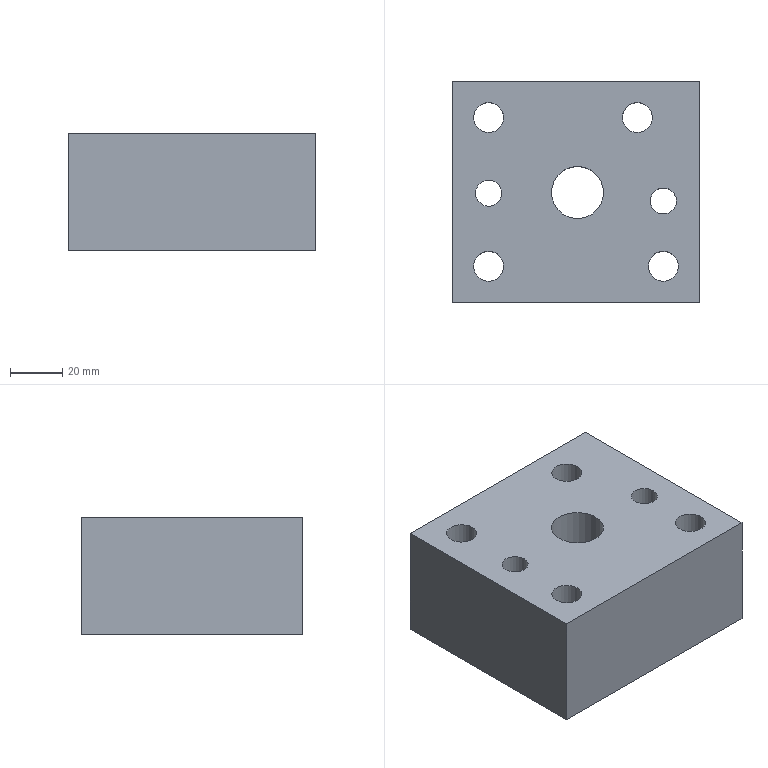Part | STEP file | lll_id4318_x_t | 1 solid | 13 faces | box 95 x 85 x 45 mm | volume 323443 mm3 | cylinder 7 | plane 6 | commonest cylinder face diameters 11.509 x4 10 x2 20 x1
STEP:
#1=CARTESIAN_POINT('',(937.935,42.75,-80.));
#2=VERTEX_POINT('',#1);
#3=CARTESIAN_POINT('',(937.935,-42.25,-80.));
#4=VERTEX_POINT('',#3);
#5=CARTESIAN_POINT('',(937.935,10.25,-80.));
#6=DIRECTION('',(0.,-1.,0.));
#7=VECTOR('',#6,1.);
#8=LINE('',#5,#7);
#9=EDGE_CURVE('',#2,#4,#8,.T.);
#10=ORIENTED_EDGE('',*,*,#9,.F.);
#11=CARTESIAN_POINT('',(937.935,42.75,-35.));
#12=VERTEX_POINT('',#11);
#13=CARTESIAN_POINT('',(937.935,42.75,-35.));
#14=DIRECTION('',(0.,0.,-1.));
#15=VECTOR('',#14,1.);
#16=LINE('',#13,#15);
#17=EDGE_CURVE('',#12,#2,#16,.T.);
#18=ORIENTED_EDGE('',*,*,#17,.F.);
#19=CARTESIAN_POINT('',(937.935,-42.25,-35.));
#20=VERTEX_POINT('',#19);
#21=CARTESIAN_POINT('',(937.935,10.25,-35.));
#22=DIRECTION('',(0.,1.,0.));
#23=VECTOR('',#22,1.);
#24=LINE('',#21,#23);
#25=EDGE_CURVE('',#20,#12,#24,.T.);
#26=ORIENTED_EDGE('',*,*,#25,.F.);
#27=CARTESIAN_POINT('',(937.935,-42.25,-35.));
#28=DIRECTION('',(0.,0.,-1.));
#29=VECTOR('',#28,1.);
#30=LINE('',#27,#29);
#31=EDGE_CURVE('',#20,#4,#30,.T.);
#32=ORIENTED_EDGE('',*,*,#31,.T.);
#33=EDGE_LOOP('',(#10,#18,#26,#32));
#34=FACE_OUTER_BOUND('',#33,.T.);
#35=CARTESIAN_POINT('',(937.935,10.25,-35.));
#36=DIRECTION('',(-1.,0.,0.));
#37=DIRECTION('',(0.,1.,0.));
#38=AXIS2_PLACEMENT_3D('',#35,#36,#37);
#39=PLANE('',#38);
#40=ADVANCED_FACE('',(#34),#39,.F.);
#41=CARTESIAN_POINT('',(842.935,-42.25,-80.));
#42=VERTEX_POINT('',#41);
#43=CARTESIAN_POINT('',(920.435,-42.25,-80.));
#44=DIRECTION('',(-1.,0.,0.));
#45=VECTOR('',#44,1.);
#46=LINE('',#43,#45);
#47=EDGE_CURVE('',#4,#42,#46,.T.);
#48=ORIENTED_EDGE('',*,*,#47,.F.);
#49=ORIENTED_EDGE('',*,*,#31,.F.);
#50=CARTESIAN_POINT('',(842.935,-42.25,-35.));
#51=VERTEX_POINT('',#50);
#52=CARTESIAN_POINT('',(920.435,-42.25,-35.));
#53=DIRECTION('',(1.,0.,0.));
#54=VECTOR('',#53,1.);
#55=LINE('',#52,#54);
#56=EDGE_CURVE('',#51,#20,#55,.T.);
#57=ORIENTED_EDGE('',*,*,#56,.F.);
#58=CARTESIAN_POINT('',(842.935,-42.25,-35.));
#59=DIRECTION('',(0.,0.,-1.));
#60=VECTOR('',#59,1.);
#61=LINE('',#58,#60);
#62=EDGE_CURVE('',#51,#42,#61,.T.);
#63=ORIENTED_EDGE('',*,*,#62,.T.);
#64=EDGE_LOOP('',(#48,#49,#57,#63));
#65=FACE_OUTER_BOUND('',#64,.T.);
#66=CARTESIAN_POINT('',(920.435,-42.25,-35.));
#67=DIRECTION('',(0.,1.,0.));
#68=DIRECTION('',(1.,0.,0.));
#69=AXIS2_PLACEMENT_3D('',#66,#67,#68);
#70=PLANE('',#69);
#71=ADVANCED_FACE('',(#65),#70,.F.);
#72=CARTESIAN_POINT('',(842.935,42.75,-80.));
#73=VERTEX_POINT('',#72);
#74=CARTESIAN_POINT('',(842.935,10.25,-80.));
#75=DIRECTION('',(0.,1.,0.));
#76=VECTOR('',#75,1.);
#77=LINE('',#74,#76);
#78=EDGE_CURVE('',#42,#73,#77,.T.);
#79=ORIENTED_EDGE('',*,*,#78,.F.);
#80=ORIENTED_EDGE('',*,*,#62,.F.);
#81=CARTESIAN_POINT('',(842.935,42.75,-35.));
#82=VERTEX_POINT('',#81);
#83=CARTESIAN_POINT('',(842.935,10.25,-35.));
#84=DIRECTION('',(0.,-1.,0.));
#85=VECTOR('',#84,1.);
#86=LINE('',#83,#85);
#87=EDGE_CURVE('',#82,#51,#86,.T.);
#88=ORIENTED_EDGE('',*,*,#87,.F.);
#89=CARTESIAN_POINT('',(842.935,42.75,-35.));
#90=DIRECTION('',(0.,0.,-1.));
#91=VECTOR('',#90,1.);
#92=LINE('',#89,#91);
#93=EDGE_CURVE('',#82,#73,#92,.T.);
#94=ORIENTED_EDGE('',*,*,#93,.T.);
#95=EDGE_LOOP('',(#79,#80,#88,#94));
#96=FACE_OUTER_BOUND('',#95,.T.);
#97=CARTESIAN_POINT('',(842.935,10.25,-35.));
#98=DIRECTION('',(1.,0.,0.));
#99=DIRECTION('',(0.,-1.,0.));
#100=AXIS2_PLACEMENT_3D('',#97,#98,#99);
#101=PLANE('',#100);
#102=ADVANCED_FACE('',(#96),#101,.F.);
#103=CARTESIAN_POINT('',(920.435,42.75,-80.));
#104=DIRECTION('',(1.,0.,0.));
#105=VECTOR('',#104,1.);
#106=LINE('',#103,#105);
#107=EDGE_CURVE('',#73,#2,#106,.T.);
#108=ORIENTED_EDGE('',*,*,#107,.F.);
#109=ORIENTED_EDGE('',*,*,#93,.F.);
#110=CARTESIAN_POINT('',(920.435,42.75,-35.));
#111=DIRECTION('',(-1.,0.,0.));
#112=VECTOR('',#111,1.);
#113=LINE('',#110,#112);
#114=EDGE_CURVE('',#12,#82,#113,.T.);
#115=ORIENTED_EDGE('',*,*,#114,.F.);
#116=ORIENTED_EDGE('',*,*,#17,.T.);
#117=EDGE_LOOP('',(#108,#109,#115,#116));
#118=FACE_OUTER_BOUND('',#117,.T.);
#119=CARTESIAN_POINT('',(920.435,42.75,-35.));
#120=DIRECTION('',(0.,-1.,0.));
#121=DIRECTION('',(-1.,0.,0.));
#122=AXIS2_PLACEMENT_3D('',#119,#120,#121);
#123=PLANE('',#122);
#124=ADVANCED_FACE('',(#118),#123,.F.);
#125=CARTESIAN_POINT('',(908.181,28.75,-80.));
#126=VERTEX_POINT('',#125);
#127=CARTESIAN_POINT('',(913.935,28.75,-80.));
#128=DIRECTION('',(0.,0.,1.));
#129=DIRECTION('',(-1.,0.,0.));
#130=AXIS2_PLACEMENT_3D('',#127,#128,#129);
#131=CIRCLE('',#130,5.755);
#132=EDGE_CURVE('',#126,#126,#131,.T.);
#133=ORIENTED_EDGE('',*,*,#132,.F.);
#134=EDGE_LOOP('',(#133));
#135=FACE_BOUND('',#134,.T.);
#136=CARTESIAN_POINT('',(919.69,28.75,-35.));
#137=VERTEX_POINT('',#136);
#138=CARTESIAN_POINT('',(913.935,28.75,-35.));
#139=DIRECTION('',(0.,0.,-1.));
#140=DIRECTION('',(1.,0.,0.));
#141=AXIS2_PLACEMENT_3D('',#138,#139,#140);
#142=CIRCLE('',#141,5.755);
#143=EDGE_CURVE('',#137,#137,#142,.T.);
#144=ORIENTED_EDGE('',*,*,#143,.F.);
#145=EDGE_LOOP('',(#144));
#146=FACE_BOUND('',#145,.T.);
#147=CARTESIAN_POINT('',(913.935,28.75,-35.));
#148=DIRECTION('',(0.,0.,-1.));
#149=DIRECTION('',(-1.,0.,0.));
#150=AXIS2_PLACEMENT_3D('',#147,#148,#149);
#151=CYLINDRICAL_SURFACE('',#150,5.755);
#152=ADVANCED_FACE('',(#135,#146),#151,.F.);
#153=CARTESIAN_POINT('',(918.181,-28.25,-80.));
#154=VERTEX_POINT('',#153);
#155=CARTESIAN_POINT('',(923.935,-28.25,-80.));
#156=DIRECTION('',(0.,0.,1.));
#157=DIRECTION('',(-1.,0.,0.));
#158=AXIS2_PLACEMENT_3D('',#155,#156,#157);
#159=CIRCLE('',#158,5.755);
#160=EDGE_CURVE('',#154,#154,#159,.T.);
#161=ORIENTED_EDGE('',*,*,#160,.F.);
#162=EDGE_LOOP('',(#161));
#163=FACE_BOUND('',#162,.T.);
#164=CARTESIAN_POINT('',(929.69,-28.25,-35.));
#165=VERTEX_POINT('',#164);
#166=CARTESIAN_POINT('',(923.935,-28.25,-35.));
#167=DIRECTION('',(0.,0.,-1.));
#168=DIRECTION('',(1.,0.,0.));
#169=AXIS2_PLACEMENT_3D('',#166,#167,#168);
#170=CIRCLE('',#169,5.755);
#171=EDGE_CURVE('',#165,#165,#170,.T.);
#172=ORIENTED_EDGE('',*,*,#171,.F.);
#173=EDGE_LOOP('',(#172));
#174=FACE_BOUND('',#173,.T.);
#175=CARTESIAN_POINT('',(923.935,-28.25,-35.));
#176=DIRECTION('',(0.,0.,-1.));
#177=DIRECTION('',(-1.,0.,0.));
#178=AXIS2_PLACEMENT_3D('',#175,#176,#177);
#179=CYLINDRICAL_SURFACE('',#178,5.755);
#180=ADVANCED_FACE('',(#163,#174),#179,.F.);
#181=CARTESIAN_POINT('',(918.935,-3.25,-80.));
#182=VERTEX_POINT('',#181);
#183=CARTESIAN_POINT('',(923.935,-3.25,-80.));
#184=DIRECTION('',(0.,0.,1.));
#185=DIRECTION('',(-1.,0.,0.));
#186=AXIS2_PLACEMENT_3D('',#183,#184,#185);
#187=CIRCLE('',#186,5.);
#188=EDGE_CURVE('',#182,#182,#187,.T.);
#189=ORIENTED_EDGE('',*,*,#188,.F.);
#190=EDGE_LOOP('',(#189));
#191=FACE_BOUND('',#190,.T.);
#192=CARTESIAN_POINT('',(928.935,-3.25,-35.));
#193=VERTEX_POINT('',#192);
#194=CARTESIAN_POINT('',(923.935,-3.25,-35.));
#195=DIRECTION('',(0.,0.,-1.));
#196=DIRECTION('',(1.,0.,0.));
#197=AXIS2_PLACEMENT_3D('',#194,#195,#196);
#198=CIRCLE('',#197,5.);
#199=EDGE_CURVE('',#193,#193,#198,.T.);
#200=ORIENTED_EDGE('',*,*,#199,.F.);
#201=EDGE_LOOP('',(#200));
#202=FACE_BOUND('',#201,.T.);
#203=CARTESIAN_POINT('',(923.935,-3.25,-35.));
#204=DIRECTION('',(0.,0.,-1.));
#205=DIRECTION('',(-1.,0.,0.));
#206=AXIS2_PLACEMENT_3D('',#203,#204,#205);
#207=CYLINDRICAL_SURFACE('',#206,5.);
#208=ADVANCED_FACE('',(#191,#202),#207,.F.);
#209=CARTESIAN_POINT('',(851.181,-28.25,-80.));
#210=VERTEX_POINT('',#209);
#211=CARTESIAN_POINT('',(856.935,-28.25,-80.));
#212=DIRECTION('',(0.,0.,1.));
#213=DIRECTION('',(-1.,0.,0.));
#214=AXIS2_PLACEMENT_3D('',#211,#212,#213);
#215=CIRCLE('',#214,5.755);
#216=EDGE_CURVE('',#210,#210,#215,.T.);
#217=ORIENTED_EDGE('',*,*,#216,.F.);
#218=EDGE_LOOP('',(#217));
#219=FACE_BOUND('',#218,.T.);
#220=CARTESIAN_POINT('',(862.69,-28.25,-35.));
#221=VERTEX_POINT('',#220);
#222=CARTESIAN_POINT('',(856.935,-28.25,-35.));
#223=DIRECTION('',(0.,0.,-1.));
#224=DIRECTION('',(1.,0.,0.));
#225=AXIS2_PLACEMENT_3D('',#222,#223,#224);
#226=CIRCLE('',#225,5.755);
#227=EDGE_CURVE('',#221,#221,#226,.T.);
#228=ORIENTED_EDGE('',*,*,#227,.F.);
#229=EDGE_LOOP('',(#228));
#230=FACE_BOUND('',#229,.T.);
#231=CARTESIAN_POINT('',(856.935,-28.25,-35.));
#232=DIRECTION('',(0.,0.,-1.));
#233=DIRECTION('',(-1.,0.,0.));
#234=AXIS2_PLACEMENT_3D('',#231,#232,#233);
#235=CYLINDRICAL_SURFACE('',#234,5.755);
#236=ADVANCED_FACE('',(#219,#230),#235,.F.);
#237=CARTESIAN_POINT('',(851.181,28.75,-80.));
#238=VERTEX_POINT('',#237);
#239=CARTESIAN_POINT('',(856.935,28.75,-80.));
#240=DIRECTION('',(0.,0.,1.));
#241=DIRECTION('',(-1.,0.,0.));
#242=AXIS2_PLACEMENT_3D('',#239,#240,#241);
#243=CIRCLE('',#242,5.755);
#244=EDGE_CURVE('',#238,#238,#243,.T.);
#245=ORIENTED_EDGE('',*,*,#244,.F.);
#246=EDGE_LOOP('',(#245));
#247=FACE_BOUND('',#246,.T.);
#248=CARTESIAN_POINT('',(862.69,28.75,-35.));
#249=VERTEX_POINT('',#248);
#250=CARTESIAN_POINT('',(856.935,28.75,-35.));
#251=DIRECTION('',(0.,0.,-1.));
#252=DIRECTION('',(1.,0.,0.));
#253=AXIS2_PLACEMENT_3D('',#250,#251,#252);
#254=CIRCLE('',#253,5.755);
#255=EDGE_CURVE('',#249,#249,#254,.T.);
#256=ORIENTED_EDGE('',*,*,#255,.F.);
#257=EDGE_LOOP('',(#256));
#258=FACE_BOUND('',#257,.T.);
#259=CARTESIAN_POINT('',(856.935,28.75,-35.));
#260=DIRECTION('',(0.,0.,-1.));
#261=DIRECTION('',(-1.,0.,0.));
#262=AXIS2_PLACEMENT_3D('',#259,#260,#261);
#263=CYLINDRICAL_SURFACE('',#262,5.755);
#264=ADVANCED_FACE('',(#247,#258),#263,.F.);
#265=CARTESIAN_POINT('',(851.935,-0.25,-80.));
#266=VERTEX_POINT('',#265);
#267=CARTESIAN_POINT('',(856.935,-0.25,-80.));
#268=DIRECTION('',(0.,0.,1.));
#269=DIRECTION('',(-1.,0.,0.));
#270=AXIS2_PLACEMENT_3D('',#267,#268,#269);
#271=CIRCLE('',#270,5.);
#272=EDGE_CURVE('',#266,#266,#271,.T.);
#273=ORIENTED_EDGE('',*,*,#272,.F.);
#274=EDGE_LOOP('',(#273));
#275=FACE_BOUND('',#274,.T.);
#276=CARTESIAN_POINT('',(861.935,-0.25,-35.));
#277=VERTEX_POINT('',#276);
#278=CARTESIAN_POINT('',(856.935,-0.25,-35.));
#279=DIRECTION('',(0.,0.,-1.));
#280=DIRECTION('',(1.,0.,0.));
#281=AXIS2_PLACEMENT_3D('',#278,#279,#280);
#282=CIRCLE('',#281,5.);
#283=EDGE_CURVE('',#277,#277,#282,.T.);
#284=ORIENTED_EDGE('',*,*,#283,.F.);
#285=EDGE_LOOP('',(#284));
#286=FACE_BOUND('',#285,.T.);
#287=CARTESIAN_POINT('',(856.935,-0.25,-35.));
#288=DIRECTION('',(0.,0.,-1.));
#289=DIRECTION('',(-1.,0.,0.));
#290=AXIS2_PLACEMENT_3D('',#287,#288,#289);
#291=CYLINDRICAL_SURFACE('',#290,5.);
#292=ADVANCED_FACE('',(#275,#286),#291,.F.);
#293=CARTESIAN_POINT('',(881.,0.,-35.));
#294=VERTEX_POINT('',#293);
#295=CARTESIAN_POINT('',(891.,0.,-35.));
#296=DIRECTION('',(0.,0.,-1.));
#297=DIRECTION('',(-1.,0.,0.));
#298=AXIS2_PLACEMENT_3D('',#295,#296,#297);
#299=CIRCLE('',#298,10.);
#300=EDGE_CURVE('',#294,#294,#299,.T.);
#301=ORIENTED_EDGE('',*,*,#300,.F.);
#302=EDGE_LOOP('',(#301));
#303=FACE_BOUND('',#302,.T.);
#304=CARTESIAN_POINT('',(881.,0.,-80.));
#305=VERTEX_POINT('',#304);
#306=CARTESIAN_POINT('',(891.,0.,-80.));
#307=DIRECTION('',(0.,0.,-1.));
#308=DIRECTION('',(-1.,0.,0.));
#309=AXIS2_PLACEMENT_3D('',#306,#307,#308);
#310=CIRCLE('',#309,10.);
#311=EDGE_CURVE('',#305,#305,#310,.T.);
#312=ORIENTED_EDGE('',*,*,#311,.T.);
#313=EDGE_LOOP('',(#312));
#314=FACE_BOUND('',#313,.T.);
#315=CARTESIAN_POINT('',(891.,0.,-35.));
#316=DIRECTION('',(0.,0.,-1.));
#317=DIRECTION('',(-1.,0.,0.));
#318=AXIS2_PLACEMENT_3D('',#315,#316,#317);
#319=CYLINDRICAL_SURFACE('',#318,10.);
#320=ADVANCED_FACE('',(#303,#314),#319,.F.);
#321=ORIENTED_EDGE('',*,*,#87,.T.);
#322=ORIENTED_EDGE('',*,*,#56,.T.);
#323=ORIENTED_EDGE('',*,*,#25,.T.);
#324=ORIENTED_EDGE('',*,*,#114,.T.);
#325=EDGE_LOOP('',(#321,#322,#323,#324));
#326=FACE_BOUND('',#325,.T.);
#327=ORIENTED_EDGE('',*,*,#143,.T.);
#328=EDGE_LOOP('',(#327));
#329=FACE_BOUND('',#328,.T.);
#330=ORIENTED_EDGE('',*,*,#171,.T.);
#331=EDGE_LOOP('',(#330));
#332=FACE_BOUND('',#331,.T.);
#333=ORIENTED_EDGE('',*,*,#199,.T.);
#334=EDGE_LOOP('',(#333));
#335=FACE_BOUND('',#334,.T.);
#336=ORIENTED_EDGE('',*,*,#227,.T.);
#337=EDGE_LOOP('',(#336));
#338=FACE_BOUND('',#337,.T.);
#339=ORIENTED_EDGE('',*,*,#255,.T.);
#340=EDGE_LOOP('',(#339));
#341=FACE_BOUND('',#340,.T.);
#342=ORIENTED_EDGE('',*,*,#283,.T.);
#343=EDGE_LOOP('',(#342));
#344=FACE_BOUND('',#343,.T.);
#345=ORIENTED_EDGE('',*,*,#300,.T.);
#346=EDGE_LOOP('',(#345));
#347=FACE_BOUND('',#346,.T.);
#348=CARTESIAN_POINT('',(920.435,25.25,-35.));
#349=DIRECTION('',(0.,0.,-1.));
#350=DIRECTION('',(1.,0.,0.));
#351=AXIS2_PLACEMENT_3D('',#348,#349,#350);
#352=PLANE('',#351);
#353=ADVANCED_FACE('',(#326,#329,#332,#335,#338,#341,#344,#347),#352,.F.);
#354=ORIENTED_EDGE('',*,*,#311,.F.);
#355=EDGE_LOOP('',(#354));
#356=FACE_BOUND('',#355,.T.);
#357=ORIENTED_EDGE('',*,*,#9,.T.);
#358=ORIENTED_EDGE('',*,*,#47,.T.);
#359=ORIENTED_EDGE('',*,*,#78,.T.);
#360=ORIENTED_EDGE('',*,*,#107,.T.);
#361=EDGE_LOOP('',(#357,#358,#359,#360));
#362=FACE_BOUND('',#361,.T.);
#363=ORIENTED_EDGE('',*,*,#132,.T.);
#364=EDGE_LOOP('',(#363));
#365=FACE_BOUND('',#364,.T.);
#366=ORIENTED_EDGE('',*,*,#160,.T.);
#367=EDGE_LOOP('',(#366));
#368=FACE_BOUND('',#367,.T.);
#369=ORIENTED_EDGE('',*,*,#188,.T.);
#370=EDGE_LOOP('',(#369));
#371=FACE_BOUND('',#370,.T.);
#372=ORIENTED_EDGE('',*,*,#216,.T.);
#373=EDGE_LOOP('',(#372));
#374=FACE_BOUND('',#373,.T.);
#375=ORIENTED_EDGE('',*,*,#244,.T.);
#376=EDGE_LOOP('',(#375));
#377=FACE_BOUND('',#376,.T.);
#378=ORIENTED_EDGE('',*,*,#272,.T.);
#379=EDGE_LOOP('',(#378));
#380=FACE_BOUND('',#379,.T.);
#381=CARTESIAN_POINT('',(890.,49.715,-80.));
#382=DIRECTION('',(0.,0.,-1.));
#383=DIRECTION('',(-1.,0.,0.));
#384=AXIS2_PLACEMENT_3D('',#381,#382,#383);
#385=PLANE('',#384);
#386=ADVANCED_FACE('',(#356,#362,#365,#368,#371,#374,#377,#380),#385,.T.);
#387=CLOSED_SHELL('',(#40,#71,#102,#124,#152,#180,#208,#236,#264,#292,#320,#353,#386));
#388=MANIFOLD_SOLID_BREP('',#387);
#389=(LENGTH_UNIT()NAMED_UNIT(*)SI_UNIT(.MILLI.,.METRE.));
#390=UNCERTAINTY_MEASURE_WITH_UNIT(LENGTH_MEASURE(0.00002),#389,'','');
#391=(NAMED_UNIT(*)PLANE_ANGLE_UNIT()SI_UNIT($,.RADIAN.));
#392=PLANE_ANGLE_MEASURE_WITH_UNIT(PLANE_ANGLE_MEASURE(0.01745),#391);
#393=DIMENSIONAL_EXPONENTS(0.,0.,0.,0.,0.,0.,0.);
#394=(CONVERSION_BASED_UNIT('DEGREE',#392)NAMED_UNIT(#393)PLANE_ANGLE_UNIT());
#395=(NAMED_UNIT(*)SI_UNIT($,.STERADIAN.)SOLID_ANGLE_UNIT());
#396=(GEOMETRIC_REPRESENTATION_CONTEXT(3)GLOBAL_UNCERTAINTY_ASSIGNED_CONTEXT((#390))GLOBAL_UNIT_ASSIGNED_CONTEXT((#389,#394,#395))REPRESENTATION_CONTEXT('',''));
#397=ADVANCED_BREP_SHAPE_REPRESENTATION('',(#388),#396);